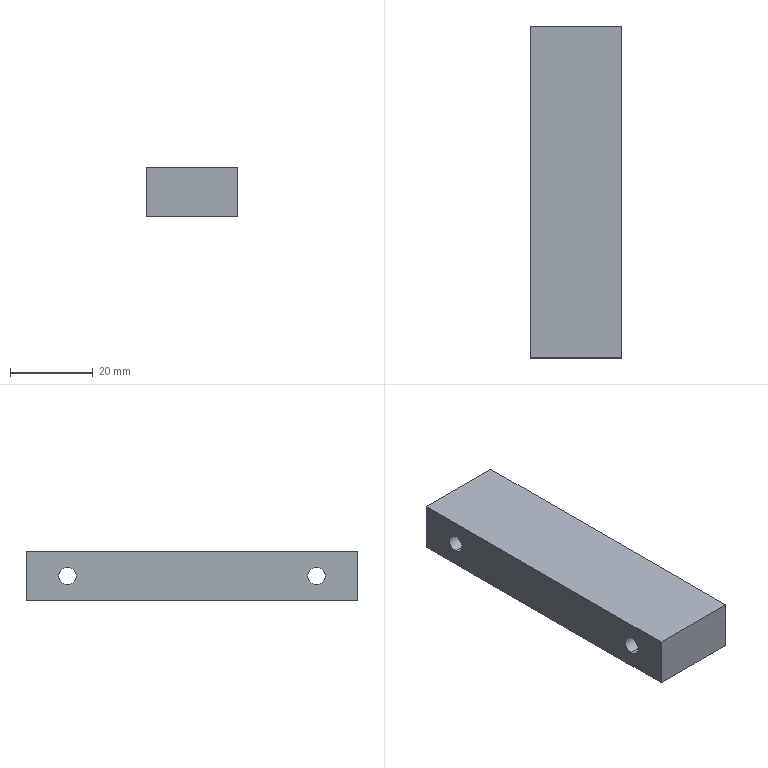Part | STEP file | CA-10-004Lift Stop Fixing Plate2_Default | 1 solid | 10 faces | box 22 x 80 x 12 mm | volume 20510 mm3 | plane 6 | cylinder 4 | commonest cylinder face diameters 4.2 x4
STEP:
#1=CARTESIAN_POINT('',(0.,0.,0.));
#2=DIRECTION('',(0.,0.,1.));
#3=DIRECTION('',(1.,0.,0.));
#4=AXIS2_PLACEMENT_3D('',#1,#2,#3);
#5=CARTESIAN_POINT('',(11.,30.,8.1));
#6=VERTEX_POINT('',#5);
#7=CARTESIAN_POINT('',(-11.,30.,8.1));
#8=VERTEX_POINT('',#7);
#9=CARTESIAN_POINT('',(-11.,30.,8.1));
#10=DIRECTION('',(-1.,0.,0.));
#11=VECTOR('',#10,1.);
#12=LINE('',#9,#11);
#13=CARTESIAN_POINT('',(-11.,30.,6.));
#14=DIRECTION('',(-1.,0.,0.));
#15=DIRECTION('',(0.,0.,1.));
#16=AXIS2_PLACEMENT_3D('',#13,#14,#15);
#17=CYLINDRICAL_SURFACE('',#16,2.1);
#18=CARTESIAN_POINT('',(6.283,0.));
#19=DIRECTION('',(0.,1.));
#20=VECTOR('',#19,1.);
#21=LINE('',#18,#20);
#22=(GEOMETRIC_REPRESENTATION_CONTEXT(2)PARAMETRIC_REPRESENTATION_CONTEXT()REPRESENTATION_CONTEXT('',''));
#23=DEFINITIONAL_REPRESENTATION('',(#21),#22);
#24=PCURVE('',#17,#23);
#25=CARTESIAN_POINT('',(-11.,30.,6.));
#26=DIRECTION('',(-1.,0.,0.));
#27=DIRECTION('',(0.,0.,1.));
#28=AXIS2_PLACEMENT_3D('',#25,#26,#27);
#29=CYLINDRICAL_SURFACE('',#28,2.1);
#30=CARTESIAN_POINT('',(0.,0.));
#31=DIRECTION('',(0.,1.));
#32=VECTOR('',#31,1.);
#33=LINE('',#30,#32);
#34=(GEOMETRIC_REPRESENTATION_CONTEXT(2)PARAMETRIC_REPRESENTATION_CONTEXT()REPRESENTATION_CONTEXT('',''));
#35=DEFINITIONAL_REPRESENTATION('',(#33),#34);
#36=PCURVE('',#29,#35);
#37=SURFACE_CURVE('',#12,(#24,#36),.PCURVE_S1.);
#38=EDGE_CURVE('',#6,#8,#37,.T.);
#39=ORIENTED_EDGE('',*,*,#38,.T.);
#40=CARTESIAN_POINT('',(-11.,30.,3.9));
#41=VERTEX_POINT('',#40);
#42=CARTESIAN_POINT('',(-11.,30.,6.));
#43=DIRECTION('',(-1.,0.,0.));
#44=DIRECTION('',(0.,0.,1.));
#45=AXIS2_PLACEMENT_3D('',#42,#43,#44);
#46=CIRCLE('',#45,2.1);
#47=CARTESIAN_POINT('',(0.,0.));
#48=DIRECTION('',(1.,0.));
#49=VECTOR('',#48,1.);
#50=LINE('',#47,#49);
#51=(GEOMETRIC_REPRESENTATION_CONTEXT(2)PARAMETRIC_REPRESENTATION_CONTEXT()REPRESENTATION_CONTEXT('',''));
#52=DEFINITIONAL_REPRESENTATION('',(#50),#51);
#53=PCURVE('',#17,#52);
#54=CARTESIAN_POINT('',(-11.,40.,12.));
#55=DIRECTION('',(1.,0.,0.));
#56=DIRECTION('',(0.,1.,0.));
#57=AXIS2_PLACEMENT_3D('',#54,#55,#56);
#58=PLANE('',#57);
#59=CARTESIAN_POINT('',(-10.,-3.9));
#60=CARTESIAN_POINT('',(-6.363,-3.9));
#61=CARTESIAN_POINT('',(-8.181,-7.05));
#62=CARTESIAN_POINT('',(-10.,-10.2));
#63=CARTESIAN_POINT('',(-11.819,-7.05));
#64=CARTESIAN_POINT('',(-13.637,-3.9));
#65=CARTESIAN_POINT('',(-10.,-3.9));
#66=(BOUNDED_CURVE()B_SPLINE_CURVE(2,(#59,#60,#61,#62,#63,#64,#65),.UNSPECIFIED.,.T.,.F.)B_SPLINE_CURVE_WITH_KNOTS((1,2,2,2,2,1),(-2.094,0.,2.094,4.189,6.283,8.378),.UNSPECIFIED.)CURVE()GEOMETRIC_REPRESENTATION_ITEM()RATIONAL_B_SPLINE_CURVE((1.,0.5,1.,0.5,1.,0.5,1.))REPRESENTATION_ITEM(''));
#67=(GEOMETRIC_REPRESENTATION_CONTEXT(2)PARAMETRIC_REPRESENTATION_CONTEXT()REPRESENTATION_CONTEXT('',''));
#68=DEFINITIONAL_REPRESENTATION('',(#66),#67);
#69=PCURVE('',#58,#68);
#70=SURFACE_CURVE('',#46,(#53,#69),.PCURVE_S1.);
#71=EDGE_CURVE('',#41,#8,#70,.T.);
#72=ORIENTED_EDGE('',*,*,#71,.F.);
#73=CARTESIAN_POINT('',(11.,30.,3.9));
#74=VERTEX_POINT('',#73);
#75=CARTESIAN_POINT('',(-11.,30.,3.9));
#76=DIRECTION('',(-1.,0.,0.));
#77=VECTOR('',#76,1.);
#78=LINE('',#75,#77);
#79=CARTESIAN_POINT('',(3.142,0.));
#80=DIRECTION('',(0.,1.));
#81=VECTOR('',#80,1.);
#82=LINE('',#79,#81);
#83=(GEOMETRIC_REPRESENTATION_CONTEXT(2)PARAMETRIC_REPRESENTATION_CONTEXT()REPRESENTATION_CONTEXT('',''));
#84=DEFINITIONAL_REPRESENTATION('',(#82),#83);
#85=PCURVE('',#17,#84);
#86=CARTESIAN_POINT('',(3.142,0.));
#87=DIRECTION('',(0.,1.));
#88=VECTOR('',#87,1.);
#89=LINE('',#86,#88);
#90=(GEOMETRIC_REPRESENTATION_CONTEXT(2)PARAMETRIC_REPRESENTATION_CONTEXT()REPRESENTATION_CONTEXT('',''));
#91=DEFINITIONAL_REPRESENTATION('',(#89),#90);
#92=PCURVE('',#29,#91);
#93=SURFACE_CURVE('',#78,(#85,#92),.PCURVE_S1.);
#94=EDGE_CURVE('',#74,#41,#93,.T.);
#95=ORIENTED_EDGE('',*,*,#94,.F.);
#96=CARTESIAN_POINT('',(11.,30.,6.));
#97=DIRECTION('',(-1.,0.,0.));
#98=DIRECTION('',(0.,0.,1.));
#99=AXIS2_PLACEMENT_3D('',#96,#97,#98);
#100=CIRCLE('',#99,2.1);
#101=CARTESIAN_POINT('',(0.,-22.));
#102=DIRECTION('',(1.,0.));
#103=VECTOR('',#102,1.);
#104=LINE('',#101,#103);
#105=(GEOMETRIC_REPRESENTATION_CONTEXT(2)PARAMETRIC_REPRESENTATION_CONTEXT()REPRESENTATION_CONTEXT('',''));
#106=DEFINITIONAL_REPRESENTATION('',(#104),#105);
#107=PCURVE('',#17,#106);
#108=CARTESIAN_POINT('',(11.,40.,12.));
#109=DIRECTION('',(-1.,0.,0.));
#110=DIRECTION('',(0.,-1.,0.));
#111=AXIS2_PLACEMENT_3D('',#108,#109,#110);
#112=PLANE('',#111);
#113=CARTESIAN_POINT('',(10.,-6.));
#114=DIRECTION('',(0.,1.));
#115=AXIS2_PLACEMENT_2D('',#113,#114);
#116=CIRCLE('',#115,2.1);
#117=(GEOMETRIC_REPRESENTATION_CONTEXT(2)PARAMETRIC_REPRESENTATION_CONTEXT()REPRESENTATION_CONTEXT('',''));
#118=DEFINITIONAL_REPRESENTATION('',(#116),#117);
#119=PCURVE('',#112,#118);
#120=SURFACE_CURVE('',#100,(#107,#119),.PCURVE_S1.);
#121=EDGE_CURVE('',#74,#6,#120,.T.);
#122=ORIENTED_EDGE('',*,*,#121,.T.);
#123=EDGE_LOOP('',(#39,#72,#95,#122));
#124=FACE_BOUND('',#123,.F.);
#125=ADVANCED_FACE('',(#124),#17,.F.);
#126=CARTESIAN_POINT('',(11.,-30.,8.1));
#127=VERTEX_POINT('',#126);
#128=CARTESIAN_POINT('',(-11.,-30.,8.1));
#129=VERTEX_POINT('',#128);
#130=CARTESIAN_POINT('',(-11.,-30.,8.1));
#131=DIRECTION('',(-1.,0.,0.));
#132=VECTOR('',#131,1.);
#133=LINE('',#130,#132);
#134=CARTESIAN_POINT('',(-11.,-30.,6.));
#135=DIRECTION('',(-1.,0.,0.));
#136=DIRECTION('',(0.,0.,1.));
#137=AXIS2_PLACEMENT_3D('',#134,#135,#136);
#138=CYLINDRICAL_SURFACE('',#137,2.1);
#139=CARTESIAN_POINT('',(6.283,0.));
#140=DIRECTION('',(0.,1.));
#141=VECTOR('',#140,1.);
#142=LINE('',#139,#141);
#143=(GEOMETRIC_REPRESENTATION_CONTEXT(2)PARAMETRIC_REPRESENTATION_CONTEXT()REPRESENTATION_CONTEXT('',''));
#144=DEFINITIONAL_REPRESENTATION('',(#142),#143);
#145=PCURVE('',#138,#144);
#146=CARTESIAN_POINT('',(-11.,-30.,6.));
#147=DIRECTION('',(-1.,0.,0.));
#148=DIRECTION('',(0.,0.,1.));
#149=AXIS2_PLACEMENT_3D('',#146,#147,#148);
#150=CYLINDRICAL_SURFACE('',#149,2.1);
#151=CARTESIAN_POINT('',(0.,0.));
#152=DIRECTION('',(0.,1.));
#153=VECTOR('',#152,1.);
#154=LINE('',#151,#153);
#155=(GEOMETRIC_REPRESENTATION_CONTEXT(2)PARAMETRIC_REPRESENTATION_CONTEXT()REPRESENTATION_CONTEXT('',''));
#156=DEFINITIONAL_REPRESENTATION('',(#154),#155);
#157=PCURVE('',#150,#156);
#158=SURFACE_CURVE('',#133,(#145,#157),.PCURVE_S1.);
#159=EDGE_CURVE('',#127,#129,#158,.T.);
#160=ORIENTED_EDGE('',*,*,#159,.T.);
#161=CARTESIAN_POINT('',(-11.,-30.,3.9));
#162=VERTEX_POINT('',#161);
#163=CARTESIAN_POINT('',(-11.,-30.,6.));
#164=DIRECTION('',(-1.,0.,0.));
#165=DIRECTION('',(0.,0.,1.));
#166=AXIS2_PLACEMENT_3D('',#163,#164,#165);
#167=CIRCLE('',#166,2.1);
#168=CARTESIAN_POINT('',(0.,0.));
#169=DIRECTION('',(1.,0.));
#170=VECTOR('',#169,1.);
#171=LINE('',#168,#170);
#172=(GEOMETRIC_REPRESENTATION_CONTEXT(2)PARAMETRIC_REPRESENTATION_CONTEXT()REPRESENTATION_CONTEXT('',''));
#173=DEFINITIONAL_REPRESENTATION('',(#171),#172);
#174=PCURVE('',#138,#173);
#175=CARTESIAN_POINT('',(-70.,-3.9));
#176=CARTESIAN_POINT('',(-66.363,-3.9));
#177=CARTESIAN_POINT('',(-68.181,-7.05));
#178=CARTESIAN_POINT('',(-70.,-10.2));
#179=CARTESIAN_POINT('',(-71.819,-7.05));
#180=CARTESIAN_POINT('',(-73.637,-3.9));
#181=CARTESIAN_POINT('',(-70.,-3.9));
#182=(BOUNDED_CURVE()B_SPLINE_CURVE(2,(#175,#176,#177,#178,#179,#180,#181),.UNSPECIFIED.,.T.,.F.)B_SPLINE_CURVE_WITH_KNOTS((1,2,2,2,2,1),(-2.094,0.,2.094,4.189,6.283,8.378),.UNSPECIFIED.)CURVE()GEOMETRIC_REPRESENTATION_ITEM()RATIONAL_B_SPLINE_CURVE((1.,0.5,1.,0.5,1.,0.5,1.))REPRESENTATION_ITEM(''));
#183=(GEOMETRIC_REPRESENTATION_CONTEXT(2)PARAMETRIC_REPRESENTATION_CONTEXT()REPRESENTATION_CONTEXT('',''));
#184=DEFINITIONAL_REPRESENTATION('',(#182),#183);
#185=PCURVE('',#58,#184);
#186=SURFACE_CURVE('',#167,(#174,#185),.PCURVE_S1.);
#187=EDGE_CURVE('',#162,#129,#186,.T.);
#188=ORIENTED_EDGE('',*,*,#187,.F.);
#189=CARTESIAN_POINT('',(11.,-30.,3.9));
#190=VERTEX_POINT('',#189);
#191=CARTESIAN_POINT('',(-11.,-30.,3.9));
#192=DIRECTION('',(-1.,0.,0.));
#193=VECTOR('',#192,1.);
#194=LINE('',#191,#193);
#195=CARTESIAN_POINT('',(3.142,0.));
#196=DIRECTION('',(0.,1.));
#197=VECTOR('',#196,1.);
#198=LINE('',#195,#197);
#199=(GEOMETRIC_REPRESENTATION_CONTEXT(2)PARAMETRIC_REPRESENTATION_CONTEXT()REPRESENTATION_CONTEXT('',''));
#200=DEFINITIONAL_REPRESENTATION('',(#198),#199);
#201=PCURVE('',#138,#200);
#202=CARTESIAN_POINT('',(3.142,0.));
#203=DIRECTION('',(0.,1.));
#204=VECTOR('',#203,1.);
#205=LINE('',#202,#204);
#206=(GEOMETRIC_REPRESENTATION_CONTEXT(2)PARAMETRIC_REPRESENTATION_CONTEXT()REPRESENTATION_CONTEXT('',''));
#207=DEFINITIONAL_REPRESENTATION('',(#205),#206);
#208=PCURVE('',#150,#207);
#209=SURFACE_CURVE('',#194,(#201,#208),.PCURVE_S1.);
#210=EDGE_CURVE('',#190,#162,#209,.T.);
#211=ORIENTED_EDGE('',*,*,#210,.F.);
#212=CARTESIAN_POINT('',(11.,-30.,6.));
#213=DIRECTION('',(-1.,0.,0.));
#214=DIRECTION('',(0.,0.,1.));
#215=AXIS2_PLACEMENT_3D('',#212,#213,#214);
#216=CIRCLE('',#215,2.1);
#217=CARTESIAN_POINT('',(0.,-22.));
#218=DIRECTION('',(1.,0.));
#219=VECTOR('',#218,1.);
#220=LINE('',#217,#219);
#221=(GEOMETRIC_REPRESENTATION_CONTEXT(2)PARAMETRIC_REPRESENTATION_CONTEXT()REPRESENTATION_CONTEXT('',''));
#222=DEFINITIONAL_REPRESENTATION('',(#220),#221);
#223=PCURVE('',#138,#222);
#224=CARTESIAN_POINT('',(70.,-6.));
#225=DIRECTION('',(0.,1.));
#226=AXIS2_PLACEMENT_2D('',#224,#225);
#227=CIRCLE('',#226,2.1);
#228=(GEOMETRIC_REPRESENTATION_CONTEXT(2)PARAMETRIC_REPRESENTATION_CONTEXT()REPRESENTATION_CONTEXT('',''));
#229=DEFINITIONAL_REPRESENTATION('',(#227),#228);
#230=PCURVE('',#112,#229);
#231=SURFACE_CURVE('',#216,(#223,#230),.PCURVE_S1.);
#232=EDGE_CURVE('',#190,#127,#231,.T.);
#233=ORIENTED_EDGE('',*,*,#232,.T.);
#234=EDGE_LOOP('',(#160,#188,#211,#233));
#235=FACE_BOUND('',#234,.F.);
#236=ADVANCED_FACE('',(#235),#138,.F.);
#237=CARTESIAN_POINT('',(11.,30.,6.));
#238=DIRECTION('',(-1.,0.,0.));
#239=DIRECTION('',(0.,0.,1.));
#240=AXIS2_PLACEMENT_3D('',#237,#238,#239);
#241=CIRCLE('',#240,2.1);
#242=CARTESIAN_POINT('',(10.,-6.));
#243=DIRECTION('',(0.,1.));
#244=AXIS2_PLACEMENT_2D('',#242,#243);
#245=CIRCLE('',#244,2.1);
#246=(GEOMETRIC_REPRESENTATION_CONTEXT(2)PARAMETRIC_REPRESENTATION_CONTEXT()REPRESENTATION_CONTEXT('',''));
#247=DEFINITIONAL_REPRESENTATION('',(#245),#246);
#248=PCURVE('',#112,#247);
#249=CARTESIAN_POINT('',(0.,-22.));
#250=DIRECTION('',(1.,0.));
#251=VECTOR('',#250,1.);
#252=LINE('',#249,#251);
#253=(GEOMETRIC_REPRESENTATION_CONTEXT(2)PARAMETRIC_REPRESENTATION_CONTEXT()REPRESENTATION_CONTEXT('',''));
#254=DEFINITIONAL_REPRESENTATION('',(#252),#253);
#255=PCURVE('',#29,#254);
#256=SURFACE_CURVE('',#241,(#248,#255),.PCURVE_S1.);
#257=EDGE_CURVE('',#6,#74,#256,.T.);
#258=ORIENTED_EDGE('',*,*,#257,.T.);
#259=ORIENTED_EDGE('',*,*,#121,.T.);
#260=EDGE_LOOP('',(#258,#259));
#261=FACE_BOUND('',#260,.T.);
#262=CARTESIAN_POINT('',(11.,-30.,6.));
#263=DIRECTION('',(-1.,0.,0.));
#264=DIRECTION('',(0.,0.,1.));
#265=AXIS2_PLACEMENT_3D('',#262,#263,#264);
#266=CIRCLE('',#265,2.1);
#267=CARTESIAN_POINT('',(70.,-6.));
#268=DIRECTION('',(0.,1.));
#269=AXIS2_PLACEMENT_2D('',#267,#268);
#270=CIRCLE('',#269,2.1);
#271=(GEOMETRIC_REPRESENTATION_CONTEXT(2)PARAMETRIC_REPRESENTATION_CONTEXT()REPRESENTATION_CONTEXT('',''));
#272=DEFINITIONAL_REPRESENTATION('',(#270),#271);
#273=PCURVE('',#112,#272);
#274=CARTESIAN_POINT('',(0.,-22.));
#275=DIRECTION('',(1.,0.));
#276=VECTOR('',#275,1.);
#277=LINE('',#274,#276);
#278=(GEOMETRIC_REPRESENTATION_CONTEXT(2)PARAMETRIC_REPRESENTATION_CONTEXT()REPRESENTATION_CONTEXT('',''));
#279=DEFINITIONAL_REPRESENTATION('',(#277),#278);
#280=PCURVE('',#150,#279);
#281=SURFACE_CURVE('',#266,(#273,#280),.PCURVE_S1.);
#282=EDGE_CURVE('',#127,#190,#281,.T.);
#283=ORIENTED_EDGE('',*,*,#282,.T.);
#284=ORIENTED_EDGE('',*,*,#232,.T.);
#285=EDGE_LOOP('',(#283,#284));
#286=FACE_BOUND('',#285,.T.);
#287=CARTESIAN_POINT('',(11.,-40.,0.));
#288=VERTEX_POINT('',#287);
#289=CARTESIAN_POINT('',(11.,40.,0.));
#290=VERTEX_POINT('',#289);
#291=CARTESIAN_POINT('',(11.,40.,0.));
#292=DIRECTION('',(0.,1.,0.));
#293=VECTOR('',#292,1.);
#294=LINE('',#291,#293);
#295=CARTESIAN_POINT('',(0.,-12.));
#296=DIRECTION('',(-1.,0.));
#297=VECTOR('',#296,1.);
#298=LINE('',#295,#297);
#299=(GEOMETRIC_REPRESENTATION_CONTEXT(2)PARAMETRIC_REPRESENTATION_CONTEXT()REPRESENTATION_CONTEXT('',''));
#300=DEFINITIONAL_REPRESENTATION('',(#298),#299);
#301=PCURVE('',#112,#300);
#302=CARTESIAN_POINT('',(0.,0.,0.));
#303=DIRECTION('',(0.,0.,1.));
#304=DIRECTION('',(1.,0.,0.));
#305=AXIS2_PLACEMENT_3D('',#302,#303,#304);
#306=PLANE('',#305);
#307=CARTESIAN_POINT('',(11.,40.));
#308=DIRECTION('',(0.,1.));
#309=VECTOR('',#308,1.);
#310=LINE('',#307,#309);
#311=(GEOMETRIC_REPRESENTATION_CONTEXT(2)PARAMETRIC_REPRESENTATION_CONTEXT()REPRESENTATION_CONTEXT('',''));
#312=DEFINITIONAL_REPRESENTATION('',(#310),#311);
#313=PCURVE('',#306,#312);
#314=SURFACE_CURVE('',#294,(#301,#313),.PCURVE_S1.);
#315=EDGE_CURVE('',#288,#290,#314,.T.);
#316=ORIENTED_EDGE('',*,*,#315,.T.);
#317=CARTESIAN_POINT('',(11.,40.,12.));
#318=VERTEX_POINT('',#317);
#319=CARTESIAN_POINT('',(11.,40.,12.));
#320=DIRECTION('',(0.,0.,-1.));
#321=VECTOR('',#320,1.);
#322=LINE('',#319,#321);
#323=CARTESIAN_POINT('',(0.,0.));
#324=DIRECTION('',(0.,-1.));
#325=VECTOR('',#324,1.);
#326=LINE('',#323,#325);
#327=(GEOMETRIC_REPRESENTATION_CONTEXT(2)PARAMETRIC_REPRESENTATION_CONTEXT()REPRESENTATION_CONTEXT('',''));
#328=DEFINITIONAL_REPRESENTATION('',(#326),#327);
#329=PCURVE('',#112,#328);
#330=CARTESIAN_POINT('',(-11.,40.,12.));
#331=DIRECTION('',(0.,-1.,0.));
#332=DIRECTION('',(0.,0.,-1.));
#333=AXIS2_PLACEMENT_3D('',#330,#331,#332);
#334=PLANE('',#333);
#335=CARTESIAN_POINT('',(0.,22.));
#336=DIRECTION('',(1.,0.));
#337=VECTOR('',#336,1.);
#338=LINE('',#335,#337);
#339=(GEOMETRIC_REPRESENTATION_CONTEXT(2)PARAMETRIC_REPRESENTATION_CONTEXT()REPRESENTATION_CONTEXT('',''));
#340=DEFINITIONAL_REPRESENTATION('',(#338),#339);
#341=PCURVE('',#334,#340);
#342=SURFACE_CURVE('',#322,(#329,#341),.PCURVE_S1.);
#343=EDGE_CURVE('',#318,#290,#342,.T.);
#344=ORIENTED_EDGE('',*,*,#343,.F.);
#345=CARTESIAN_POINT('',(11.,-40.,12.));
#346=VERTEX_POINT('',#345);
#347=CARTESIAN_POINT('',(11.,40.,12.));
#348=DIRECTION('',(0.,1.,0.));
#349=VECTOR('',#348,1.);
#350=LINE('',#347,#349);
#351=CARTESIAN_POINT('',(0.,0.));
#352=DIRECTION('',(-1.,0.));
#353=VECTOR('',#352,1.);
#354=LINE('',#351,#353);
#355=(GEOMETRIC_REPRESENTATION_CONTEXT(2)PARAMETRIC_REPRESENTATION_CONTEXT()REPRESENTATION_CONTEXT('',''));
#356=DEFINITIONAL_REPRESENTATION('',(#354),#355);
#357=PCURVE('',#112,#356);
#358=CARTESIAN_POINT('',(0.,0.,12.));
#359=DIRECTION('',(0.,0.,1.));
#360=DIRECTION('',(1.,0.,0.));
#361=AXIS2_PLACEMENT_3D('',#358,#359,#360);
#362=PLANE('',#361);
#363=CARTESIAN_POINT('',(11.,40.));
#364=DIRECTION('',(0.,1.));
#365=VECTOR('',#364,1.);
#366=LINE('',#363,#365);
#367=(GEOMETRIC_REPRESENTATION_CONTEXT(2)PARAMETRIC_REPRESENTATION_CONTEXT()REPRESENTATION_CONTEXT('',''));
#368=DEFINITIONAL_REPRESENTATION('',(#366),#367);
#369=PCURVE('',#362,#368);
#370=SURFACE_CURVE('',#350,(#357,#369),.PCURVE_S1.);
#371=EDGE_CURVE('',#346,#318,#370,.T.);
#372=ORIENTED_EDGE('',*,*,#371,.F.);
#373=CARTESIAN_POINT('',(11.,-40.,12.));
#374=DIRECTION('',(0.,0.,-1.));
#375=VECTOR('',#374,1.);
#376=LINE('',#373,#375);
#377=CARTESIAN_POINT('',(80.,0.));
#378=DIRECTION('',(0.,-1.));
#379=VECTOR('',#378,1.);
#380=LINE('',#377,#379);
#381=(GEOMETRIC_REPRESENTATION_CONTEXT(2)PARAMETRIC_REPRESENTATION_CONTEXT()REPRESENTATION_CONTEXT('',''));
#382=DEFINITIONAL_REPRESENTATION('',(#380),#381);
#383=PCURVE('',#112,#382);
#384=CARTESIAN_POINT('',(-11.,-40.,12.));
#385=DIRECTION('',(0.,1.,0.));
#386=DIRECTION('',(0.,0.,1.));
#387=AXIS2_PLACEMENT_3D('',#384,#385,#386);
#388=PLANE('',#387);
#389=CARTESIAN_POINT('',(0.,22.));
#390=DIRECTION('',(-1.,0.));
#391=VECTOR('',#390,1.);
#392=LINE('',#389,#391);
#393=(GEOMETRIC_REPRESENTATION_CONTEXT(2)PARAMETRIC_REPRESENTATION_CONTEXT()REPRESENTATION_CONTEXT('',''));
#394=DEFINITIONAL_REPRESENTATION('',(#392),#393);
#395=PCURVE('',#388,#394);
#396=SURFACE_CURVE('',#376,(#383,#395),.PCURVE_S1.);
#397=EDGE_CURVE('',#346,#288,#396,.T.);
#398=ORIENTED_EDGE('',*,*,#397,.T.);
#399=EDGE_LOOP('',(#316,#344,#372,#398));
#400=FACE_BOUND('',#399,.T.);
#401=ADVANCED_FACE('',(#261,#286,#400),#112,.F.);
#402=CARTESIAN_POINT('',(-11.,40.,0.));
#403=VERTEX_POINT('',#402);
#404=CARTESIAN_POINT('',(-11.,40.,0.));
#405=DIRECTION('',(-1.,0.,0.));
#406=VECTOR('',#405,1.);
#407=LINE('',#404,#406);
#408=CARTESIAN_POINT('',(12.,0.));
#409=DIRECTION('',(0.,-1.));
#410=VECTOR('',#409,1.);
#411=LINE('',#408,#410);
#412=(GEOMETRIC_REPRESENTATION_CONTEXT(2)PARAMETRIC_REPRESENTATION_CONTEXT()REPRESENTATION_CONTEXT('',''));
#413=DEFINITIONAL_REPRESENTATION('',(#411),#412);
#414=PCURVE('',#334,#413);
#415=CARTESIAN_POINT('',(-11.,40.));
#416=DIRECTION('',(-1.,0.));
#417=VECTOR('',#416,1.);
#418=LINE('',#415,#417);
#419=(GEOMETRIC_REPRESENTATION_CONTEXT(2)PARAMETRIC_REPRESENTATION_CONTEXT()REPRESENTATION_CONTEXT('',''));
#420=DEFINITIONAL_REPRESENTATION('',(#418),#419);
#421=PCURVE('',#306,#420);
#422=SURFACE_CURVE('',#407,(#414,#421),.PCURVE_S1.);
#423=EDGE_CURVE('',#290,#403,#422,.T.);
#424=ORIENTED_EDGE('',*,*,#423,.T.);
#425=CARTESIAN_POINT('',(-11.,40.,12.));
#426=VERTEX_POINT('',#425);
#427=CARTESIAN_POINT('',(-11.,40.,12.));
#428=DIRECTION('',(0.,0.,-1.));
#429=VECTOR('',#428,1.);
#430=LINE('',#427,#429);
#431=CARTESIAN_POINT('',(0.,0.));
#432=DIRECTION('',(1.,0.));
#433=VECTOR('',#432,1.);
#434=LINE('',#431,#433);
#435=(GEOMETRIC_REPRESENTATION_CONTEXT(2)PARAMETRIC_REPRESENTATION_CONTEXT()REPRESENTATION_CONTEXT('',''));
#436=DEFINITIONAL_REPRESENTATION('',(#434),#435);
#437=PCURVE('',#334,#436);
#438=CARTESIAN_POINT('',(0.,0.));
#439=DIRECTION('',(0.,-1.));
#440=VECTOR('',#439,1.);
#441=LINE('',#438,#440);
#442=(GEOMETRIC_REPRESENTATION_CONTEXT(2)PARAMETRIC_REPRESENTATION_CONTEXT()REPRESENTATION_CONTEXT('',''));
#443=DEFINITIONAL_REPRESENTATION('',(#441),#442);
#444=PCURVE('',#58,#443);
#445=SURFACE_CURVE('',#430,(#437,#444),.PCURVE_S1.);
#446=EDGE_CURVE('',#426,#403,#445,.T.);
#447=ORIENTED_EDGE('',*,*,#446,.F.);
#448=CARTESIAN_POINT('',(-11.,40.,12.));
#449=DIRECTION('',(-1.,0.,0.));
#450=VECTOR('',#449,1.);
#451=LINE('',#448,#450);
#452=CARTESIAN_POINT('',(0.,0.));
#453=DIRECTION('',(0.,-1.));
#454=VECTOR('',#453,1.);
#455=LINE('',#452,#454);
#456=(GEOMETRIC_REPRESENTATION_CONTEXT(2)PARAMETRIC_REPRESENTATION_CONTEXT()REPRESENTATION_CONTEXT('',''));
#457=DEFINITIONAL_REPRESENTATION('',(#455),#456);
#458=PCURVE('',#334,#457);
#459=CARTESIAN_POINT('',(-11.,40.));
#460=DIRECTION('',(-1.,0.));
#461=VECTOR('',#460,1.);
#462=LINE('',#459,#461);
#463=(GEOMETRIC_REPRESENTATION_CONTEXT(2)PARAMETRIC_REPRESENTATION_CONTEXT()REPRESENTATION_CONTEXT('',''));
#464=DEFINITIONAL_REPRESENTATION('',(#462),#463);
#465=PCURVE('',#362,#464);
#466=SURFACE_CURVE('',#451,(#458,#465),.PCURVE_S1.);
#467=EDGE_CURVE('',#318,#426,#466,.T.);
#468=ORIENTED_EDGE('',*,*,#467,.F.);
#469=ORIENTED_EDGE('',*,*,#343,.T.);
#470=EDGE_LOOP('',(#424,#447,#468,#469));
#471=FACE_BOUND('',#470,.T.);
#472=ADVANCED_FACE('',(#471),#334,.F.);
#473=CARTESIAN_POINT('',(-11.,30.,6.));
#474=DIRECTION('',(-1.,0.,0.));
#475=DIRECTION('',(0.,0.,1.));
#476=AXIS2_PLACEMENT_3D('',#473,#474,#475);
#477=CIRCLE('',#476,2.1);
#478=CARTESIAN_POINT('',(-10.,-3.9));
#479=CARTESIAN_POINT('',(-6.363,-3.9));
#480=CARTESIAN_POINT('',(-8.181,-7.05));
#481=CARTESIAN_POINT('',(-10.,-10.2));
#482=CARTESIAN_POINT('',(-11.819,-7.05));
#483=CARTESIAN_POINT('',(-13.637,-3.9));
#484=CARTESIAN_POINT('',(-10.,-3.9));
#485=(BOUNDED_CURVE()B_SPLINE_CURVE(2,(#478,#479,#480,#481,#482,#483,#484),.UNSPECIFIED.,.T.,.F.)B_SPLINE_CURVE_WITH_KNOTS((1,2,2,2,2,1),(-2.094,0.,2.094,4.189,6.283,8.378),.UNSPECIFIED.)CURVE()GEOMETRIC_REPRESENTATION_ITEM()RATIONAL_B_SPLINE_CURVE((1.,0.5,1.,0.5,1.,0.5,1.))REPRESENTATION_ITEM(''));
#486=(GEOMETRIC_REPRESENTATION_CONTEXT(2)PARAMETRIC_REPRESENTATION_CONTEXT()REPRESENTATION_CONTEXT('',''));
#487=DEFINITIONAL_REPRESENTATION('',(#485),#486);
#488=PCURVE('',#58,#487);
#489=CARTESIAN_POINT('',(0.,0.));
#490=DIRECTION('',(1.,0.));
#491=VECTOR('',#490,1.);
#492=LINE('',#489,#491);
#493=(GEOMETRIC_REPRESENTATION_CONTEXT(2)PARAMETRIC_REPRESENTATION_CONTEXT()REPRESENTATION_CONTEXT('',''));
#494=DEFINITIONAL_REPRESENTATION('',(#492),#493);
#495=PCURVE('',#29,#494);
#496=SURFACE_CURVE('',#477,(#488,#495),.PCURVE_S1.);
#497=EDGE_CURVE('',#8,#41,#496,.T.);
#498=ORIENTED_EDGE('',*,*,#497,.F.);
#499=ORIENTED_EDGE('',*,*,#71,.F.);
#500=EDGE_LOOP('',(#498,#499));
#501=FACE_BOUND('',#500,.T.);
#502=CARTESIAN_POINT('',(-11.,-30.,6.));
#503=DIRECTION('',(-1.,0.,0.));
#504=DIRECTION('',(0.,0.,1.));
#505=AXIS2_PLACEMENT_3D('',#502,#503,#504);
#506=CIRCLE('',#505,2.1);
#507=CARTESIAN_POINT('',(-70.,-3.9));
#508=CARTESIAN_POINT('',(-66.363,-3.9));
#509=CARTESIAN_POINT('',(-68.181,-7.05));
#510=CARTESIAN_POINT('',(-70.,-10.2));
#511=CARTESIAN_POINT('',(-71.819,-7.05));
#512=CARTESIAN_POINT('',(-73.637,-3.9));
#513=CARTESIAN_POINT('',(-70.,-3.9));
#514=(BOUNDED_CURVE()B_SPLINE_CURVE(2,(#507,#508,#509,#510,#511,#512,#513),.UNSPECIFIED.,.T.,.F.)B_SPLINE_CURVE_WITH_KNOTS((1,2,2,2,2,1),(-2.094,0.,2.094,4.189,6.283,8.378),.UNSPECIFIED.)CURVE()GEOMETRIC_REPRESENTATION_ITEM()RATIONAL_B_SPLINE_CURVE((1.,0.5,1.,0.5,1.,0.5,1.))REPRESENTATION_ITEM(''));
#515=(GEOMETRIC_REPRESENTATION_CONTEXT(2)PARAMETRIC_REPRESENTATION_CONTEXT()REPRESENTATION_CONTEXT('',''));
#516=DEFINITIONAL_REPRESENTATION('',(#514),#515);
#517=PCURVE('',#58,#516);
#518=CARTESIAN_POINT('',(0.,0.));
#519=DIRECTION('',(1.,0.));
#520=VECTOR('',#519,1.);
#521=LINE('',#518,#520);
#522=(GEOMETRIC_REPRESENTATION_CONTEXT(2)PARAMETRIC_REPRESENTATION_CONTEXT()REPRESENTATION_CONTEXT('',''));
#523=DEFINITIONAL_REPRESENTATION('',(#521),#522);
#524=PCURVE('',#150,#523);
#525=SURFACE_CURVE('',#506,(#517,#524),.PCURVE_S1.);
#526=EDGE_CURVE('',#129,#162,#525,.T.);
#527=ORIENTED_EDGE('',*,*,#526,.F.);
#528=ORIENTED_EDGE('',*,*,#187,.F.);
#529=EDGE_LOOP('',(#527,#528));
#530=FACE_BOUND('',#529,.T.);
#531=CARTESIAN_POINT('',(-11.,-40.,0.));
#532=VERTEX_POINT('',#531);
#533=CARTESIAN_POINT('',(-11.,40.,0.));
#534=DIRECTION('',(0.,-1.,0.));
#535=VECTOR('',#534,1.);
#536=LINE('',#533,#535);
#537=CARTESIAN_POINT('',(0.,-12.));
#538=DIRECTION('',(-1.,0.));
#539=VECTOR('',#538,1.);
#540=LINE('',#537,#539);
#541=(GEOMETRIC_REPRESENTATION_CONTEXT(2)PARAMETRIC_REPRESENTATION_CONTEXT()REPRESENTATION_CONTEXT('',''));
#542=DEFINITIONAL_REPRESENTATION('',(#540),#541);
#543=PCURVE('',#58,#542);
#544=CARTESIAN_POINT('',(-11.,40.));
#545=DIRECTION('',(0.,-1.));
#546=VECTOR('',#545,1.);
#547=LINE('',#544,#546);
#548=(GEOMETRIC_REPRESENTATION_CONTEXT(2)PARAMETRIC_REPRESENTATION_CONTEXT()REPRESENTATION_CONTEXT('',''));
#549=DEFINITIONAL_REPRESENTATION('',(#547),#548);
#550=PCURVE('',#306,#549);
#551=SURFACE_CURVE('',#536,(#543,#550),.PCURVE_S1.);
#552=EDGE_CURVE('',#403,#532,#551,.T.);
#553=ORIENTED_EDGE('',*,*,#552,.T.);
#554=CARTESIAN_POINT('',(-11.,-40.,12.));
#555=VERTEX_POINT('',#554);
#556=CARTESIAN_POINT('',(-11.,-40.,12.));
#557=DIRECTION('',(0.,0.,-1.));
#558=VECTOR('',#557,1.);
#559=LINE('',#556,#558);
#560=CARTESIAN_POINT('',(-80.,0.));
#561=DIRECTION('',(0.,-1.));
#562=VECTOR('',#561,1.);
#563=LINE('',#560,#562);
#564=(GEOMETRIC_REPRESENTATION_CONTEXT(2)PARAMETRIC_REPRESENTATION_CONTEXT()REPRESENTATION_CONTEXT('',''));
#565=DEFINITIONAL_REPRESENTATION('',(#563),#564);
#566=PCURVE('',#58,#565);
#567=CARTESIAN_POINT('',(0.,0.));
#568=DIRECTION('',(-1.,0.));
#569=VECTOR('',#568,1.);
#570=LINE('',#567,#569);
#571=(GEOMETRIC_REPRESENTATION_CONTEXT(2)PARAMETRIC_REPRESENTATION_CONTEXT()REPRESENTATION_CONTEXT('',''));
#572=DEFINITIONAL_REPRESENTATION('',(#570),#571);
#573=PCURVE('',#388,#572);
#574=SURFACE_CURVE('',#559,(#566,#573),.PCURVE_S1.);
#575=EDGE_CURVE('',#555,#532,#574,.T.);
#576=ORIENTED_EDGE('',*,*,#575,.F.);
#577=CARTESIAN_POINT('',(-11.,40.,12.));
#578=DIRECTION('',(0.,-1.,0.));
#579=VECTOR('',#578,1.);
#580=LINE('',#577,#579);
#581=CARTESIAN_POINT('',(0.,0.));
#582=DIRECTION('',(-1.,0.));
#583=VECTOR('',#582,1.);
#584=LINE('',#581,#583);
#585=(GEOMETRIC_REPRESENTATION_CONTEXT(2)PARAMETRIC_REPRESENTATION_CONTEXT()REPRESENTATION_CONTEXT('',''));
#586=DEFINITIONAL_REPRESENTATION('',(#584),#585);
#587=PCURVE('',#58,#586);
#588=CARTESIAN_POINT('',(-11.,40.));
#589=DIRECTION('',(0.,-1.));
#590=VECTOR('',#589,1.);
#591=LINE('',#588,#590);
#592=(GEOMETRIC_REPRESENTATION_CONTEXT(2)PARAMETRIC_REPRESENTATION_CONTEXT()REPRESENTATION_CONTEXT('',''));
#593=DEFINITIONAL_REPRESENTATION('',(#591),#592);
#594=PCURVE('',#362,#593);
#595=SURFACE_CURVE('',#580,(#587,#594),.PCURVE_S1.);
#596=EDGE_CURVE('',#426,#555,#595,.T.);
#597=ORIENTED_EDGE('',*,*,#596,.F.);
#598=ORIENTED_EDGE('',*,*,#446,.T.);
#599=EDGE_LOOP('',(#553,#576,#597,#598));
#600=FACE_BOUND('',#599,.T.);
#601=ADVANCED_FACE('',(#501,#530,#600),#58,.F.);
#602=CARTESIAN_POINT('',(-11.,-40.,0.));
#603=DIRECTION('',(1.,0.,0.));
#604=VECTOR('',#603,1.);
#605=LINE('',#602,#604);
#606=CARTESIAN_POINT('',(-12.,0.));
#607=DIRECTION('',(0.,1.));
#608=VECTOR('',#607,1.);
#609=LINE('',#606,#608);
#610=(GEOMETRIC_REPRESENTATION_CONTEXT(2)PARAMETRIC_REPRESENTATION_CONTEXT()REPRESENTATION_CONTEXT('',''));
#611=DEFINITIONAL_REPRESENTATION('',(#609),#610);
#612=PCURVE('',#388,#611);
#613=CARTESIAN_POINT('',(-11.,-40.));
#614=DIRECTION('',(1.,0.));
#615=VECTOR('',#614,1.);
#616=LINE('',#613,#615);
#617=(GEOMETRIC_REPRESENTATION_CONTEXT(2)PARAMETRIC_REPRESENTATION_CONTEXT()REPRESENTATION_CONTEXT('',''));
#618=DEFINITIONAL_REPRESENTATION('',(#616),#617);
#619=PCURVE('',#306,#618);
#620=SURFACE_CURVE('',#605,(#612,#619),.PCURVE_S1.);
#621=EDGE_CURVE('',#532,#288,#620,.T.);
#622=ORIENTED_EDGE('',*,*,#621,.T.);
#623=ORIENTED_EDGE('',*,*,#397,.F.);
#624=CARTESIAN_POINT('',(-11.,-40.,12.));
#625=DIRECTION('',(1.,0.,0.));
#626=VECTOR('',#625,1.);
#627=LINE('',#624,#626);
#628=CARTESIAN_POINT('',(0.,0.));
#629=DIRECTION('',(0.,1.));
#630=VECTOR('',#629,1.);
#631=LINE('',#628,#630);
#632=(GEOMETRIC_REPRESENTATION_CONTEXT(2)PARAMETRIC_REPRESENTATION_CONTEXT()REPRESENTATION_CONTEXT('',''));
#633=DEFINITIONAL_REPRESENTATION('',(#631),#632);
#634=PCURVE('',#388,#633);
#635=CARTESIAN_POINT('',(-11.,-40.));
#636=DIRECTION('',(1.,0.));
#637=VECTOR('',#636,1.);
#638=LINE('',#635,#637);
#639=(GEOMETRIC_REPRESENTATION_CONTEXT(2)PARAMETRIC_REPRESENTATION_CONTEXT()REPRESENTATION_CONTEXT('',''));
#640=DEFINITIONAL_REPRESENTATION('',(#638),#639);
#641=PCURVE('',#362,#640);
#642=SURFACE_CURVE('',#627,(#634,#641),.PCURVE_S1.);
#643=EDGE_CURVE('',#555,#346,#642,.T.);
#644=ORIENTED_EDGE('',*,*,#643,.F.);
#645=ORIENTED_EDGE('',*,*,#575,.T.);
#646=EDGE_LOOP('',(#622,#623,#644,#645));
#647=FACE_BOUND('',#646,.T.);
#648=ADVANCED_FACE('',(#647),#388,.F.);
#649=ORIENTED_EDGE('',*,*,#371,.T.);
#650=ORIENTED_EDGE('',*,*,#467,.T.);
#651=ORIENTED_EDGE('',*,*,#596,.T.);
#652=ORIENTED_EDGE('',*,*,#643,.T.);
#653=EDGE_LOOP('',(#649,#650,#651,#652));
#654=FACE_BOUND('',#653,.T.);
#655=ADVANCED_FACE('',(#654),#362,.T.);
#656=ORIENTED_EDGE('',*,*,#315,.F.);
#657=ORIENTED_EDGE('',*,*,#621,.F.);
#658=ORIENTED_EDGE('',*,*,#552,.F.);
#659=ORIENTED_EDGE('',*,*,#423,.F.);
#660=EDGE_LOOP('',(#656,#657,#658,#659));
#661=FACE_BOUND('',#660,.T.);
#662=ADVANCED_FACE('',(#661),#306,.F.);
#663=ORIENTED_EDGE('',*,*,#526,.F.);
#664=ORIENTED_EDGE('',*,*,#159,.F.);
#665=ORIENTED_EDGE('',*,*,#282,.T.);
#666=ORIENTED_EDGE('',*,*,#210,.T.);
#667=EDGE_LOOP('',(#663,#664,#665,#666));
#668=FACE_BOUND('',#667,.F.);
#669=ADVANCED_FACE('',(#668),#150,.F.);
#670=ORIENTED_EDGE('',*,*,#497,.F.);
#671=ORIENTED_EDGE('',*,*,#38,.F.);
#672=ORIENTED_EDGE('',*,*,#257,.T.);
#673=ORIENTED_EDGE('',*,*,#94,.T.);
#674=EDGE_LOOP('',(#670,#671,#672,#673));
#675=FACE_BOUND('',#674,.F.);
#676=ADVANCED_FACE('',(#675),#29,.F.);
#677=CLOSED_SHELL('',(#125,#236,#401,#472,#601,#648,#655,#662,#669,#676));
#678=MANIFOLD_SOLID_BREP('',#677);
#679=(LENGTH_UNIT()NAMED_UNIT(*)SI_UNIT(.MILLI.,.METRE.));
#680=UNCERTAINTY_MEASURE_WITH_UNIT(LENGTH_MEASURE(0.0000001),#679,'','');
#681=(NAMED_UNIT(*)PLANE_ANGLE_UNIT()SI_UNIT($,.RADIAN.));
#682=(NAMED_UNIT(*)SI_UNIT($,.STERADIAN.)SOLID_ANGLE_UNIT());
#683=(GEOMETRIC_REPRESENTATION_CONTEXT(3)GLOBAL_UNCERTAINTY_ASSIGNED_CONTEXT((#680))GLOBAL_UNIT_ASSIGNED_CONTEXT((#679,#681,#682))REPRESENTATION_CONTEXT('',''));
#684=ADVANCED_BREP_SHAPE_REPRESENTATION('',(#4,#678),#683);